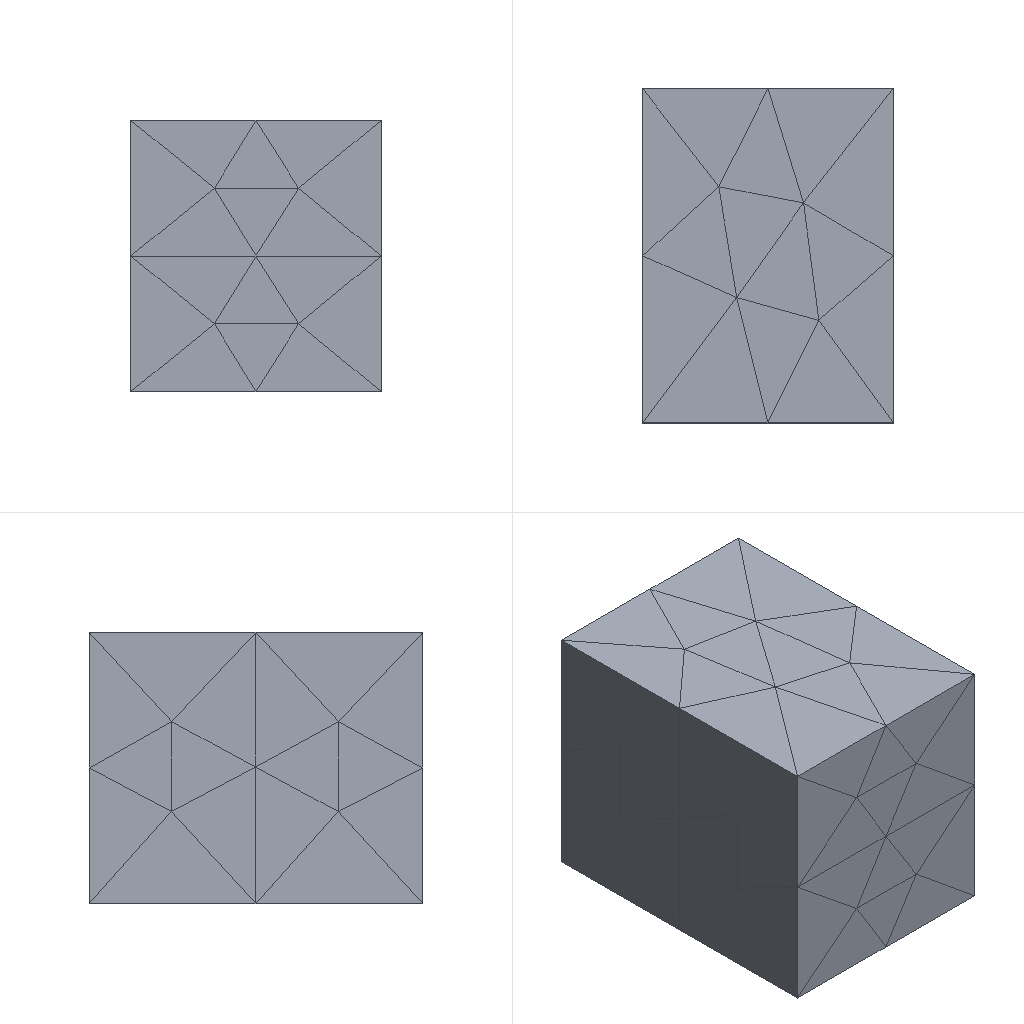Simulation study | ansys mapdl
Set-up summary:
category,name,step,type,value,unit,region
solver,ansys_mapdl
units,mm-N-s-tonne (MPa),,inferred,E=210000 density=
analysis,model,,static
mesh,nodes,,,266
mesh,elements,,,121
element_type,SOLID187,,,121
material,mat 1,,E,210000
material,mat 1,,nu,0.3
load,,model,body load temp,,,all
load,,model,force,"1000 [dir=(0, 0, -1) n=94]",,node list
bc,,model,fixed,"[dofs=UX,UY,UZ n=375]",,node list
Ansys APDL input file, long lists of numbers shortened:
/COM,ANSYS RELEASE 2026 R1           BUILD 26.1      UP20260202       09:09:39
/PREP7
/NOPR
/TITLE,2
ANTYPE, 0
*IF,_CDRDOFF,EQ,1,THEN     !if solid model was read in
_CDRDOFF=             !reset flag, numoffs already performed
*ELSE              !offset database for the following FE model
NUMOFF,NODE,      266
NUMOFF,ELEM,      121
NUMOFF,MAT ,        1
NUMOFF,TYPE,        1
*ENDIF
*SET,_RETURN ,  0.
*SET,_STATUS ,  0.
*SET,_UIQR   ,  94.
*SET,__FLOATPARAMETER__,  266.
DOF,DELETE
ETBLOCK,        1,        1
(2i9,19a9)
        1      187        0        0        0        0        0        0        0        0        0        0        0        0        0        0        0        0        0        0        0
       -1
NBLOCK,6,SOLID,       266,       266
(3i9,6e21.13e3)
        1        0        0 4.1000000000000E+001 8.0000000000000E+000
! (265 more lines like these left out)
N,UNBL,LOC,       -1,
EBLOCK,19,SOLID,       121,       121
(19i10)
         1         1         1         1         0         0         0         0        10         0         1       136       187       135       188       189       190       112       191
! (241 more lines like these left out)
        -1
MPTEMP,UNBL, 1, 1,  0.    ,
MPDATA,UNBL, 1,EX  ,       1, 1,  210000.000    ,
MPTEMP,UNBL, 1, 1,  0.    ,
MPDATA,UNBL, 1,NUXY,       1, 1, 0.3    ,
MPTEMP,UNBL, 1, 1,  0.    ,
MPDATA,UNBL, 1,PRXY,       1, 1, 0.3    ,
EXTOPT,ATTR,      0,      0,      0
EXTOPT,ESIZE,  0,  0.
EXTOPT,ACLEAR,      0
TREF,  0.
IRLF,  0
BFUNIF,TEMP,_TINY
ACEL,  0.    ,  0.    ,  0.
OMEGA,  0.    ,  0.    ,  0.
DOMEGA,  0.    ,  0.    ,  0.
CGLOC,  0.    ,  0.    ,  0.
CGOMEGA,  0.    ,  0.    ,  0.
DCGOMG,  0.    ,  0.    ,  0.
KUSE,     0
TIME,  0.
ALPHAD,  0.
BETAD,  0.
DMPRAT,  0.
DMPSTR,  0.
CRPLIM, 0.1    ,   0
CRPLIM,  0.    ,   1
NCNV,     0, 1.000000000E+12,     0,  0.    ,  0.
NEQIT,     0
ERESX,DEFA
DBLOCK,       375
(i9,a6,2(pg16.9))
        1  UX    0.00000000      0.00000000
! (374 more lines like these left out)
       -1
FBLOCK,        94
(i9,a6,2(pg16.9))
       38  FZ   -10.6382979      0.00000000
! (93 more lines like these left out)
       -1
/GO
FINISH
Results summary:
result,analysis_type_db,,,static,unstated
result,n_sets,,,1,unstated
result,load_steps[0].set,load_step=1,,1,unstated
result,load_steps[0].substep,load_step=1,,1,unstated
result,load_steps[0].time,load_step=1,,1,unstated
result,load_steps[0].freq,load_step=1,,1,unstated
result,load_steps[0].max_usum,load_step=1,,0.0004217,unstated
result,load_steps[0].max_seqv,load_step=1,,8.357,unstated
result,load_steps[0].reaction_sum.FX,load_step=1,,1.70752e-11,unstated
result,load_steps[0].reaction_sum.FY,load_step=1,,1.05378e-11,unstated
result,load_steps[0].reaction_sum.FZ,load_step=1,,1000,unstated
result,load_steps[0].reaction_sum.MX,load_step=1,,0,unstated
result,load_steps[0].reaction_sum.MY,load_step=1,,0,unstated
result,load_steps[0].reaction_sum.MZ,load_step=1,,0,unstated
result,convergence,,,results present for all listed sets,unstated